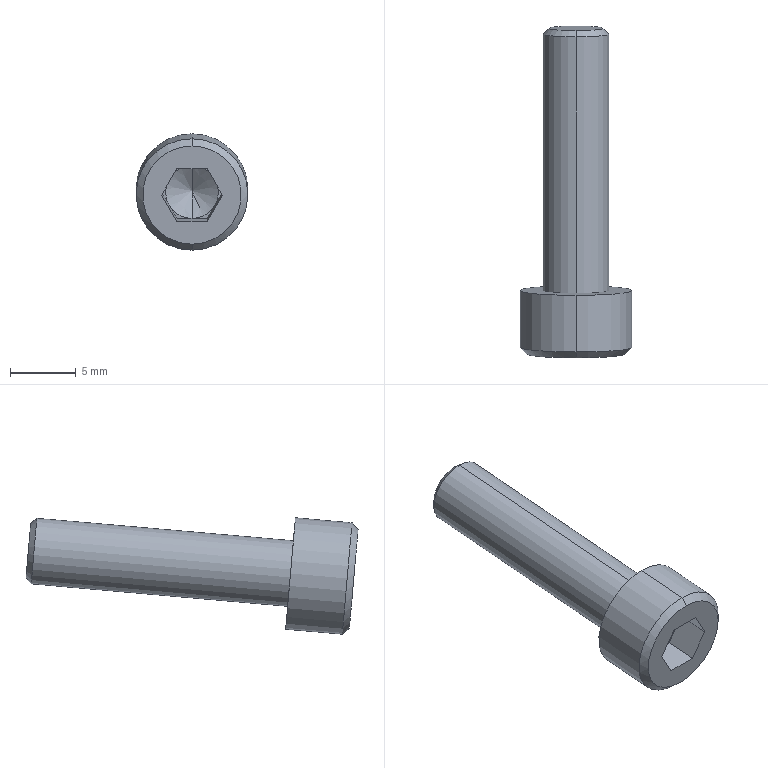Part | STEP file | 0243_Z_MCSLC40-10-16_2 | 1 solid | 25 faces | box 8.5 x 25.233 x 8.844 mm | volume 622.138 mm3 | plane 15 | cone 6 | cylinder 4 | commonest cylinder face diameters 5 x2 8.5 x2